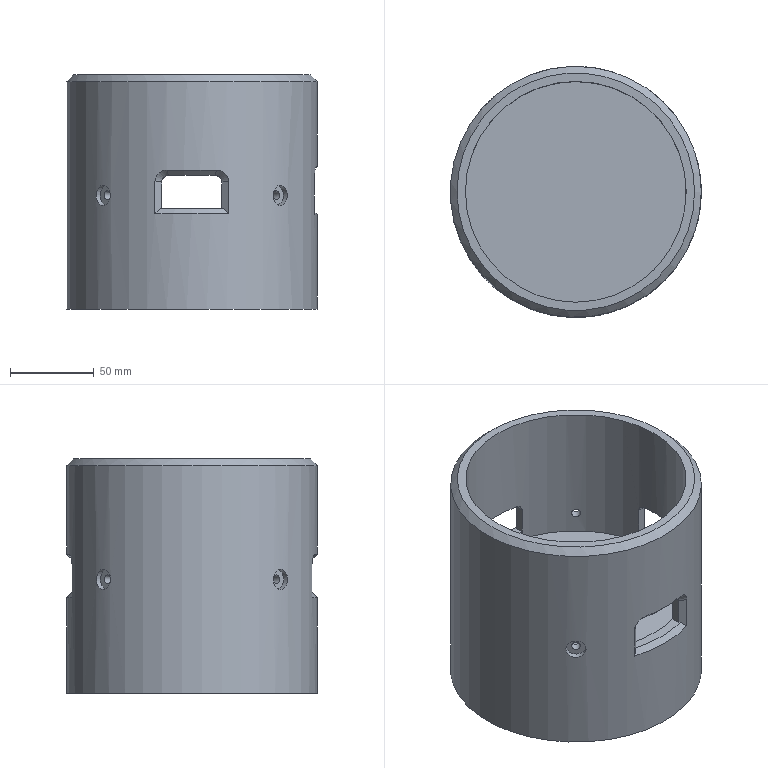Part | NX | features BREP 1 | 1 solid | 54 faces | box 150 x 150 x 140 mm | volume 1285184 mm3 | plane 25 | spline 12 | cylinder 10 | cone 7 | commonest cylinder face diameters 5.294 x4 12 x4 132 x1 150 x1